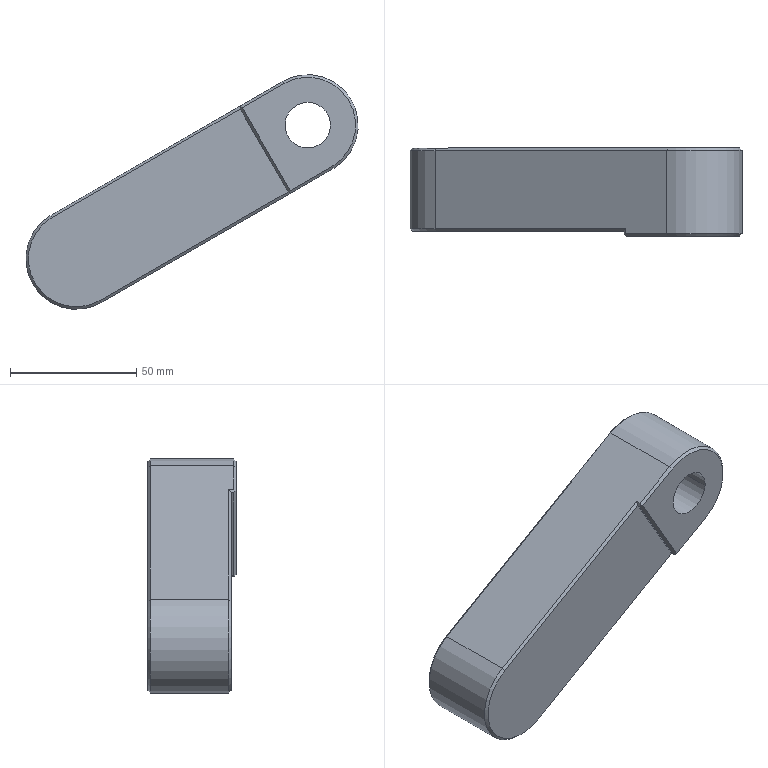Part | Creo | 1 solid | 26 faces | box 131.799 x 35 x 93 mm | volume 169707 mm3 | plane 16 | cylinder 6 | cone 4 | commonest cylinder face diameters 18.05 x2 26 x2 40 x2
STEP:
#1=CARTESIAN_POINT('',(-32.067,331.995,-173.29));
#2=VERTEX_POINT('',#1);
#3=CARTESIAN_POINT('',(-32.067,347.995,-173.29));
#4=VERTEX_POINT('',#3);
#5=CARTESIAN_POINT('',(-32.067,331.995,-173.29));
#6=DIRECTION('',(0.,1.,0.));
#7=VECTOR('',#6,16.);
#8=LINE('',#5,#7);
#9=EDGE_CURVE('',#2,#4,#8,.T.);
#10=ORIENTED_EDGE('',*,*,#9,.T.);
#11=CARTESIAN_POINT('',(-14.085,347.995,-174.863));
#12=VERTEX_POINT('',#11);
#13=CARTESIAN_POINT('',(-23.076,347.995,-174.076));
#14=DIRECTION('',(0.,-1.,0.));
#15=DIRECTION('',(-0.9962,0.,0.08716));
#16=AXIS2_PLACEMENT_3D('',#13,#14,#15);
#17=CIRCLE('',#16,9.025);
#18=EDGE_CURVE('',#4,#12,#17,.T.);
#19=ORIENTED_EDGE('',*,*,#18,.T.);
#20=CARTESIAN_POINT('',(-14.085,331.995,-174.863));
#21=VERTEX_POINT('',#20);
#22=CARTESIAN_POINT('',(-14.085,347.995,-174.863));
#23=DIRECTION('',(0.,-1.,0.));
#24=VECTOR('',#23,16.);
#25=LINE('',#22,#24);
#26=EDGE_CURVE('',#12,#21,#25,.T.);
#27=ORIENTED_EDGE('',*,*,#26,.T.);
#28=CARTESIAN_POINT('',(-23.076,331.995,-174.076));
#29=DIRECTION('',(0.,1.,0.));
#30=DIRECTION('',(0.9962,0.,-0.08716));
#31=AXIS2_PLACEMENT_3D('',#28,#29,#30);
#32=CIRCLE('',#31,9.025);
#33=EDGE_CURVE('',#21,#2,#32,.T.);
#34=ORIENTED_EDGE('',*,*,#33,.T.);
#35=EDGE_LOOP('',(#10,#19,#27,#34));
#36=FACE_OUTER_BOUND('',#35,.F.);
#37=CARTESIAN_POINT('',(-23.076,366.995,-174.076));
#38=DIRECTION('',(0.,1.,0.));
#39=DIRECTION('',(-0.9962,0.,0.08716));
#40=AXIS2_PLACEMENT_3D('',#37,#38,#39);
#41=CYLINDRICAL_SURFACE('',#40,9.025);
#42=ADVANCED_FACE('',(#36),#41,.F.);
#43=ORIENTED_EDGE('',*,*,#26,.F.);
#44=CARTESIAN_POINT('',(-23.076,347.995,-174.076));
#45=DIRECTION('',(0.,-1.,0.));
#46=DIRECTION('',(0.9962,0.,-0.08716));
#47=AXIS2_PLACEMENT_3D('',#44,#45,#46);
#48=CIRCLE('',#47,9.025);
#49=EDGE_CURVE('',#12,#4,#48,.T.);
#50=ORIENTED_EDGE('',*,*,#49,.T.);
#51=ORIENTED_EDGE('',*,*,#9,.F.);
#52=CARTESIAN_POINT('',(-23.076,331.995,-174.076));
#53=DIRECTION('',(0.,1.,0.));
#54=DIRECTION('',(-0.9962,0.,0.08716));
#55=AXIS2_PLACEMENT_3D('',#52,#53,#54);
#56=CIRCLE('',#55,9.025);
#57=EDGE_CURVE('',#2,#21,#56,.T.);
#58=ORIENTED_EDGE('',*,*,#57,.T.);
#59=EDGE_LOOP('',(#43,#50,#51,#58));
#60=FACE_OUTER_BOUND('',#59,.F.);
#61=CARTESIAN_POINT('',(-23.076,366.995,-174.076));
#62=DIRECTION('',(0.,1.,0.));
#63=DIRECTION('',(-0.9962,0.,0.08716));
#64=AXIS2_PLACEMENT_3D('',#61,#62,#63);
#65=CYLINDRICAL_SURFACE('',#64,9.025);
#66=ADVANCED_FACE('',(#60),#65,.F.);
#67=CARTESIAN_POINT('',(-10.126,347.995,-175.209));
#68=VERTEX_POINT('',#67);
#69=CARTESIAN_POINT('',(-36.027,347.995,-172.943));
#70=VERTEX_POINT('',#69);
#71=CARTESIAN_POINT('',(-23.076,347.995,-174.076));
#72=DIRECTION('',(0.,1.,0.));
#73=DIRECTION('',(0.9962,0.,-0.08716));
#74=AXIS2_PLACEMENT_3D('',#71,#72,#73);
#75=CIRCLE('',#74,13.);
#76=EDGE_CURVE('',#68,#70,#75,.T.);
#77=ORIENTED_EDGE('',*,*,#76,.F.);
#78=CARTESIAN_POINT('',(-23.076,347.995,-174.076));
#79=DIRECTION('',(0.,1.,0.));
#80=DIRECTION('',(-0.9962,0.,0.08716));
#81=AXIS2_PLACEMENT_3D('',#78,#79,#80);
#82=CIRCLE('',#81,13.);
#83=EDGE_CURVE('',#70,#68,#82,.T.);
#84=ORIENTED_EDGE('',*,*,#83,.F.);
#85=EDGE_LOOP('',(#77,#84));
#86=FACE_OUTER_BOUND('',#85,.F.);
#87=ORIENTED_EDGE('',*,*,#18,.F.);
#88=ORIENTED_EDGE('',*,*,#49,.F.);
#89=EDGE_LOOP('',(#87,#88));
#90=FACE_BOUND('',#89,.F.);
#91=CARTESIAN_POINT('',(-167.611,347.995,-30.602));
#92=DIRECTION('',(0.,1.,0.));
#93=DIRECTION('',(-0.9962,0.,0.08716));
#94=AXIS2_PLACEMENT_3D('',#91,#92,#93);
#95=PLANE('',#94);
#96=ADVANCED_FACE('',(#86,#90),#95,.T.);
#97=CARTESIAN_POINT('',(-36.027,366.995,-172.943));
#98=VERTEX_POINT('',#97);
#99=CARTESIAN_POINT('',(-36.027,347.995,-172.943));
#100=DIRECTION('',(0.,1.,0.));
#101=VECTOR('',#100,19.);
#102=LINE('',#99,#101);
#103=EDGE_CURVE('',#70,#98,#102,.T.);
#104=ORIENTED_EDGE('',*,*,#103,.T.);
#105=CARTESIAN_POINT('',(-10.126,366.995,-175.209));
#106=VERTEX_POINT('',#105);
#107=CARTESIAN_POINT('',(-23.076,366.995,-174.076));
#108=DIRECTION('',(0.,-1.,0.));
#109=DIRECTION('',(-0.9962,0.,0.08716));
#110=AXIS2_PLACEMENT_3D('',#107,#108,#109);
#111=CIRCLE('',#110,13.);
#112=EDGE_CURVE('',#98,#106,#111,.T.);
#113=ORIENTED_EDGE('',*,*,#112,.T.);
#114=CARTESIAN_POINT('',(-10.126,366.995,-175.209));
#115=DIRECTION('',(0.,-1.,0.));
#116=VECTOR('',#115,19.);
#117=LINE('',#114,#116);
#118=EDGE_CURVE('',#106,#68,#117,.T.);
#119=ORIENTED_EDGE('',*,*,#118,.T.);
#120=ORIENTED_EDGE('',*,*,#76,.T.);
#121=EDGE_LOOP('',(#104,#113,#119,#120));
#122=FACE_OUTER_BOUND('',#121,.F.);
#123=CARTESIAN_POINT('',(-23.076,366.995,-174.076));
#124=DIRECTION('',(0.,1.,0.));
#125=DIRECTION('',(-0.9962,0.,0.08716));
#126=AXIS2_PLACEMENT_3D('',#123,#124,#125);
#127=CYLINDRICAL_SURFACE('',#126,13.);
#128=ADVANCED_FACE('',(#122),#127,.F.);
#129=ORIENTED_EDGE('',*,*,#118,.F.);
#130=CARTESIAN_POINT('',(-23.076,366.995,-174.076));
#131=DIRECTION('',(0.,-1.,0.));
#132=DIRECTION('',(0.9962,0.,-0.08716));
#133=AXIS2_PLACEMENT_3D('',#130,#131,#132);
#134=CIRCLE('',#133,13.);
#135=EDGE_CURVE('',#106,#98,#134,.T.);
#136=ORIENTED_EDGE('',*,*,#135,.T.);
#137=ORIENTED_EDGE('',*,*,#103,.F.);
#138=ORIENTED_EDGE('',*,*,#83,.T.);
#139=EDGE_LOOP('',(#129,#136,#137,#138));
#140=FACE_OUTER_BOUND('',#139,.F.);
#141=CARTESIAN_POINT('',(-23.076,366.995,-174.076));
#142=DIRECTION('',(0.,1.,0.));
#143=DIRECTION('',(-0.9962,0.,0.08716));
#144=AXIS2_PLACEMENT_3D('',#141,#142,#143);
#145=CYLINDRICAL_SURFACE('',#144,13.);
#146=ADVANCED_FACE('',(#140),#145,.F.);
#147=CARTESIAN_POINT('',(-124.375,366.995,-210.622));
#148=VERTEX_POINT('',#147);
#149=CARTESIAN_POINT('',(-32.576,366.995,-157.622));
#150=VERTEX_POINT('',#149);
#151=CARTESIAN_POINT('',(-124.375,366.995,-210.622));
#152=DIRECTION('',(0.866,0.,0.5));
#153=VECTOR('',#152,106.);
#154=LINE('',#151,#153);
#155=EDGE_CURVE('',#148,#150,#154,.T.);
#156=ORIENTED_EDGE('',*,*,#155,.F.);
#157=CARTESIAN_POINT('',(-119.792,366.995,-245.429));
#158=VERTEX_POINT('',#157);
#159=CARTESIAN_POINT('',(-114.875,366.995,-227.076));
#160=DIRECTION('',(0.,1.,0.));
#161=DIRECTION('',(-0.2588,0.,-0.9659));
#162=AXIS2_PLACEMENT_3D('',#159,#160,#161);
#163=CIRCLE('',#162,19.);
#164=EDGE_CURVE('',#158,#148,#163,.T.);
#165=ORIENTED_EDGE('',*,*,#164,.F.);
#166=CARTESIAN_POINT('',(-116.531,366.995,-246.004));
#167=VERTEX_POINT('',#166);
#168=CARTESIAN_POINT('',(-114.875,366.995,-227.076));
#169=DIRECTION('',(0.,1.,0.));
#170=DIRECTION('',(-0.08716,0.,-0.9962));
#171=AXIS2_PLACEMENT_3D('',#168,#169,#170);
#172=CIRCLE('',#171,19.);
#173=EDGE_CURVE('',#167,#158,#172,.T.);
#174=ORIENTED_EDGE('',*,*,#173,.F.);
#175=CARTESIAN_POINT('',(-105.375,366.995,-243.531));
#176=VERTEX_POINT('',#175);
#177=CARTESIAN_POINT('',(-114.875,366.995,-227.076));
#178=DIRECTION('',(0.,1.,0.));
#179=DIRECTION('',(0.5,0.,-0.866));
#180=AXIS2_PLACEMENT_3D('',#177,#178,#179);
#181=CIRCLE('',#180,19.);
#182=EDGE_CURVE('',#176,#167,#181,.T.);
#183=ORIENTED_EDGE('',*,*,#182,.F.);
#184=CARTESIAN_POINT('',(-13.576,366.995,-190.531));
#185=VERTEX_POINT('',#184);
#186=CARTESIAN_POINT('',(-13.576,366.995,-190.531));
#187=DIRECTION('',(-0.866,0.,-0.5));
#188=VECTOR('',#187,106.);
#189=LINE('',#186,#188);
#190=EDGE_CURVE('',#185,#176,#189,.T.);
#191=ORIENTED_EDGE('',*,*,#190,.F.);
#192=CARTESIAN_POINT('',(-21.42,366.995,-155.148));
#193=VERTEX_POINT('',#192);
#194=CARTESIAN_POINT('',(-23.076,366.995,-174.076));
#195=DIRECTION('',(0.,1.,0.));
#196=DIRECTION('',(0.08716,0.,0.9962));
#197=AXIS2_PLACEMENT_3D('',#194,#195,#196);
#198=CIRCLE('',#197,19.);
#199=EDGE_CURVE('',#193,#185,#198,.T.);
#200=ORIENTED_EDGE('',*,*,#199,.F.);
#201=CARTESIAN_POINT('',(-23.076,366.995,-174.076));
#202=DIRECTION('',(0.,1.,0.));
#203=DIRECTION('',(-0.5,0.,0.866));
#204=AXIS2_PLACEMENT_3D('',#201,#202,#203);
#205=CIRCLE('',#204,19.);
#206=EDGE_CURVE('',#150,#193,#205,.T.);
#207=ORIENTED_EDGE('',*,*,#206,.F.);
#208=EDGE_LOOP('',(#156,#165,#174,#183,#191,#200,#207));
#209=FACE_OUTER_BOUND('',#208,.F.);
#210=ORIENTED_EDGE('',*,*,#112,.F.);
#211=ORIENTED_EDGE('',*,*,#135,.F.);
#212=EDGE_LOOP('',(#210,#211));
#213=FACE_BOUND('',#212,.F.);
#214=CARTESIAN_POINT('',(-167.611,366.995,-30.602));
#215=DIRECTION('',(0.,1.,0.));
#216=DIRECTION('',(-0.9962,0.,0.08716));
#217=AXIS2_PLACEMENT_3D('',#214,#215,#216);
#218=PLANE('',#217);
#219=ADVANCED_FACE('',(#209,#213),#218,.T.);
#220=CARTESIAN_POINT('',(-124.875,365.995,-209.756));
#221=VERTEX_POINT('',#220);
#222=CARTESIAN_POINT('',(-124.875,365.995,-209.756));
#223=DIRECTION('',(0.3536,0.7071,-0.6124));
#224=VECTOR('',#223,1.414);
#225=LINE('',#222,#224);
#226=EDGE_CURVE('',#221,#148,#225,.T.);
#227=ORIENTED_EDGE('',*,*,#226,.T.);
#228=ORIENTED_EDGE('',*,*,#155,.T.);
#229=CARTESIAN_POINT('',(-33.076,365.995,-156.756));
#230=VERTEX_POINT('',#229);
#231=CARTESIAN_POINT('',(-32.576,366.995,-157.622));
#232=DIRECTION('',(-0.3536,-0.7071,0.6124));
#233=VECTOR('',#232,1.414);
#234=LINE('',#231,#233);
#235=EDGE_CURVE('',#150,#230,#234,.T.);
#236=ORIENTED_EDGE('',*,*,#235,.T.);
#237=CARTESIAN_POINT('',(-33.076,365.995,-156.756));
#238=DIRECTION('',(-0.866,0.,-0.5));
#239=VECTOR('',#238,106.);
#240=LINE('',#237,#239);
#241=EDGE_CURVE('',#230,#221,#240,.T.);
#242=ORIENTED_EDGE('',*,*,#241,.T.);
#243=EDGE_LOOP('',(#227,#228,#236,#242));
#244=FACE_OUTER_BOUND('',#243,.F.);
#245=CARTESIAN_POINT('',(-89.118,366.495,-189.689));
#246=DIRECTION('',(-0.3536,0.7071,0.6124));
#247=DIRECTION('',(-0.3536,-0.7071,0.6124));
#248=AXIS2_PLACEMENT_3D('',#245,#246,#247);
#249=PLANE('',#248);
#250=ADVANCED_FACE('',(#244),#249,.T.);
#251=CARTESIAN_POINT('',(-104.875,365.995,-244.397));
#252=VERTEX_POINT('',#251);
#253=CARTESIAN_POINT('',(-105.375,366.995,-243.531));
#254=DIRECTION('',(0.3536,-0.7071,-0.6124));
#255=VECTOR('',#254,1.414);
#256=LINE('',#253,#255);
#257=EDGE_CURVE('',#176,#252,#256,.T.);
#258=ORIENTED_EDGE('',*,*,#257,.F.);
#259=ORIENTED_EDGE('',*,*,#182,.T.);
#260=ORIENTED_EDGE('',*,*,#173,.T.);
#261=ORIENTED_EDGE('',*,*,#164,.T.);
#262=ORIENTED_EDGE('',*,*,#226,.F.);
#263=CARTESIAN_POINT('',(-134.799,365.995,-225.333));
#264=VERTEX_POINT('',#263);
#265=CARTESIAN_POINT('',(-114.875,365.995,-227.076));
#266=DIRECTION('',(0.,1.,0.));
#267=DIRECTION('',(-0.9962,0.,0.08716));
#268=AXIS2_PLACEMENT_3D('',#265,#266,#267);
#269=CIRCLE('',#268,20.);
#270=EDGE_CURVE('',#264,#221,#269,.T.);
#271=ORIENTED_EDGE('',*,*,#270,.F.);
#272=CARTESIAN_POINT('',(-116.618,365.995,-247.));
#273=VERTEX_POINT('',#272);
#274=CARTESIAN_POINT('',(-114.875,365.995,-227.076));
#275=DIRECTION('',(0.,1.,0.));
#276=DIRECTION('',(-0.08716,0.,-0.9962));
#277=AXIS2_PLACEMENT_3D('',#274,#275,#276);
#278=CIRCLE('',#277,20.);
#279=EDGE_CURVE('',#273,#264,#278,.T.);
#280=ORIENTED_EDGE('',*,*,#279,.F.);
#281=CARTESIAN_POINT('',(-114.875,365.995,-227.076));
#282=DIRECTION('',(0.,1.,0.));
#283=DIRECTION('',(0.5,0.,-0.866));
#284=AXIS2_PLACEMENT_3D('',#281,#282,#283);
#285=CIRCLE('',#284,20.);
#286=EDGE_CURVE('',#252,#273,#285,.T.);
#287=ORIENTED_EDGE('',*,*,#286,.F.);
#288=EDGE_LOOP('',(#258,#259,#260,#261,#262,#271,#280,#287));
#289=FACE_OUTER_BOUND('',#288,.F.);
#290=CARTESIAN_POINT('',(-114.875,366.495,-227.076));
#291=DIRECTION('',(0.,-1.,0.));
#292=DIRECTION('',(-0.08716,0.,-0.9962));
#293=AXIS2_PLACEMENT_3D('',#290,#291,#292);
#294=CONICAL_SURFACE('',#293,19.5,45.);
#295=ADVANCED_FACE('',(#289),#294,.T.);
#296=CARTESIAN_POINT('',(-13.076,365.995,-191.397));
#297=VERTEX_POINT('',#296);
#298=CARTESIAN_POINT('',(-13.076,365.995,-191.397));
#299=DIRECTION('',(-0.3536,0.7071,0.6124));
#300=VECTOR('',#299,1.414);
#301=LINE('',#298,#300);
#302=EDGE_CURVE('',#297,#185,#301,.T.);
#303=ORIENTED_EDGE('',*,*,#302,.T.);
#304=ORIENTED_EDGE('',*,*,#190,.T.);
#305=ORIENTED_EDGE('',*,*,#257,.T.);
#306=CARTESIAN_POINT('',(-104.875,365.995,-244.397));
#307=DIRECTION('',(0.866,0.,0.5));
#308=VECTOR('',#307,106.);
#309=LINE('',#306,#308);
#310=EDGE_CURVE('',#252,#297,#309,.T.);
#311=ORIENTED_EDGE('',*,*,#310,.T.);
#312=EDGE_LOOP('',(#303,#304,#305,#311));
#313=FACE_OUTER_BOUND('',#312,.F.);
#314=CARTESIAN_POINT('',(-69.618,366.495,-223.464));
#315=DIRECTION('',(0.3536,0.7071,-0.6124));
#316=DIRECTION('',(0.3536,-0.7071,-0.6124));
#317=AXIS2_PLACEMENT_3D('',#314,#315,#316);
#318=PLANE('',#317);
#319=ADVANCED_FACE('',(#313),#318,.T.);
#320=ORIENTED_EDGE('',*,*,#235,.F.);
#321=ORIENTED_EDGE('',*,*,#206,.T.);
#322=ORIENTED_EDGE('',*,*,#199,.T.);
#323=ORIENTED_EDGE('',*,*,#302,.F.);
#324=CARTESIAN_POINT('',(-3.152,365.995,-175.819));
#325=VERTEX_POINT('',#324);
#326=CARTESIAN_POINT('',(-23.076,365.995,-174.076));
#327=DIRECTION('',(0.,1.,0.));
#328=DIRECTION('',(0.9962,0.,-0.08716));
#329=AXIS2_PLACEMENT_3D('',#326,#327,#328);
#330=CIRCLE('',#329,20.);
#331=EDGE_CURVE('',#325,#297,#330,.T.);
#332=ORIENTED_EDGE('',*,*,#331,.F.);
#333=CARTESIAN_POINT('',(-21.333,365.995,-154.152));
#334=VERTEX_POINT('',#333);
#335=CARTESIAN_POINT('',(-23.076,365.995,-174.076));
#336=DIRECTION('',(0.,1.,0.));
#337=DIRECTION('',(0.08716,0.,0.9962));
#338=AXIS2_PLACEMENT_3D('',#335,#336,#337);
#339=CIRCLE('',#338,20.);
#340=EDGE_CURVE('',#334,#325,#339,.T.);
#341=ORIENTED_EDGE('',*,*,#340,.F.);
#342=CARTESIAN_POINT('',(-23.076,365.995,-174.076));
#343=DIRECTION('',(0.,1.,0.));
#344=DIRECTION('',(-0.5,0.,0.866));
#345=AXIS2_PLACEMENT_3D('',#342,#343,#344);
#346=CIRCLE('',#345,20.);
#347=EDGE_CURVE('',#230,#334,#346,.T.);
#348=ORIENTED_EDGE('',*,*,#347,.F.);
#349=EDGE_LOOP('',(#320,#321,#322,#323,#332,#341,#348));
#350=FACE_OUTER_BOUND('',#349,.F.);
#351=CARTESIAN_POINT('',(-23.076,366.495,-174.076));
#352=DIRECTION('',(0.,-1.,0.));
#353=DIRECTION('',(-0.08716,0.,-0.9962));
#354=AXIS2_PLACEMENT_3D('',#351,#352,#353);
#355=CONICAL_SURFACE('',#354,19.5,45.);
#356=ADVANCED_FACE('',(#350),#355,.T.);
#357=CARTESIAN_POINT('',(-13.076,332.995,-191.397));
#358=VERTEX_POINT('',#357);
#359=CARTESIAN_POINT('',(-13.076,332.995,-191.397));
#360=DIRECTION('',(0.000000003,1.,0.000000002));
#361=VECTOR('',#360,33.);
#362=LINE('',#359,#361);
#363=EDGE_CURVE('',#358,#297,#362,.T.);
#364=ORIENTED_EDGE('',*,*,#363,.F.);
#365=CARTESIAN_POINT('',(-3.152,332.995,-175.819));
#366=VERTEX_POINT('',#365);
#367=CARTESIAN_POINT('',(-23.076,332.995,-174.076));
#368=DIRECTION('',(0.,-1.,0.));
#369=DIRECTION('',(0.5,0.,-0.866));
#370=AXIS2_PLACEMENT_3D('',#367,#368,#369);
#371=CIRCLE('',#370,20.);
#372=EDGE_CURVE('',#358,#366,#371,.T.);
#373=ORIENTED_EDGE('',*,*,#372,.T.);
#374=CARTESIAN_POINT('',(-21.333,332.995,-154.152));
#375=VERTEX_POINT('',#374);
#376=CARTESIAN_POINT('',(-23.076,332.995,-174.076));
#377=DIRECTION('',(0.,-1.,0.));
#378=DIRECTION('',(0.9962,0.,-0.08716));
#379=AXIS2_PLACEMENT_3D('',#376,#377,#378);
#380=CIRCLE('',#379,20.);
#381=EDGE_CURVE('',#366,#375,#380,.T.);
#382=ORIENTED_EDGE('',*,*,#381,.T.);
#383=CARTESIAN_POINT('',(-33.076,332.995,-156.756));
#384=VERTEX_POINT('',#383);
#385=CARTESIAN_POINT('',(-23.076,332.995,-174.076));
#386=DIRECTION('',(0.,-1.,0.));
#387=DIRECTION('',(0.08716,0.,0.9962));
#388=AXIS2_PLACEMENT_3D('',#385,#386,#387);
#389=CIRCLE('',#388,20.);
#390=EDGE_CURVE('',#375,#384,#389,.T.);
#391=ORIENTED_EDGE('',*,*,#390,.T.);
#392=CARTESIAN_POINT('',(-33.076,365.995,-156.756));
#393=DIRECTION('',(-0.000000004,-1.,-0.000000002));
#394=VECTOR('',#393,33.);
#395=LINE('',#392,#394);
#396=EDGE_CURVE('',#230,#384,#395,.T.);
#397=ORIENTED_EDGE('',*,*,#396,.F.);
#398=ORIENTED_EDGE('',*,*,#347,.T.);
#399=ORIENTED_EDGE('',*,*,#340,.T.);
#400=ORIENTED_EDGE('',*,*,#331,.T.);
#401=EDGE_LOOP('',(#364,#373,#382,#391,#397,#398,#399,#400));
#402=FACE_OUTER_BOUND('',#401,.F.);
#403=CARTESIAN_POINT('',(-23.076,331.995,-174.076));
#404=DIRECTION('',(0.,1.,0.));
#405=DIRECTION('',(-0.9962,0.,0.08716));
#406=AXIS2_PLACEMENT_3D('',#403,#404,#405);
#407=CYLINDRICAL_SURFACE('',#406,20.);
#408=ADVANCED_FACE('',(#402),#407,.T.);
#409=CARTESIAN_POINT('',(-104.875,334.995,-244.397));
#410=VERTEX_POINT('',#409);
#411=CARTESIAN_POINT('',(-104.875,365.995,-244.397));
#412=DIRECTION('',(0.,-1.,0.));
#413=VECTOR('',#412,31.);
#414=LINE('',#411,#413);
#415=EDGE_CURVE('',#252,#410,#414,.T.);
#416=ORIENTED_EDGE('',*,*,#415,.T.);
#417=CARTESIAN_POINT('',(-29.531,334.995,-200.897));
#418=VERTEX_POINT('',#417);
#419=CARTESIAN_POINT('',(-104.875,334.995,-244.397));
#420=DIRECTION('',(0.866,0.,0.5));
#421=VECTOR('',#420,87.);
#422=LINE('',#419,#421);
#423=EDGE_CURVE('',#410,#418,#422,.T.);
#424=ORIENTED_EDGE('',*,*,#423,.T.);
#425=CARTESIAN_POINT('',(-29.531,332.995,-200.897));
#426=VERTEX_POINT('',#425);
#427=CARTESIAN_POINT('',(-29.531,334.995,-200.897));
#428=DIRECTION('',(0.,-1.,0.));
#429=VECTOR('',#428,2.);
#430=LINE('',#427,#429);
#431=EDGE_CURVE('',#418,#426,#430,.T.);
#432=ORIENTED_EDGE('',*,*,#431,.T.);
#433=CARTESIAN_POINT('',(-13.076,332.995,-191.397));
#434=DIRECTION('',(-0.866,0.,-0.5));
#435=VECTOR('',#434,19.);
#436=LINE('',#433,#435);
#437=EDGE_CURVE('',#358,#426,#436,.T.);
#438=ORIENTED_EDGE('',*,*,#437,.F.);
#439=ORIENTED_EDGE('',*,*,#363,.T.);
#440=ORIENTED_EDGE('',*,*,#310,.F.);
#441=EDGE_LOOP('',(#416,#424,#432,#438,#439,#440));
#442=FACE_OUTER_BOUND('',#441,.F.);
#443=CARTESIAN_POINT('',(-13.076,331.995,-191.397));
#444=DIRECTION('',(0.5,0.,-0.866));
#445=DIRECTION('',(-0.866,0.,-0.5));
#446=AXIS2_PLACEMENT_3D('',#443,#444,#445);
#447=PLANE('',#446);
#448=ADVANCED_FACE('',(#442),#447,.T.);
#449=CARTESIAN_POINT('',(-124.875,334.995,-209.756));
#450=VERTEX_POINT('',#449);
#451=CARTESIAN_POINT('',(-124.875,334.995,-209.756));
#452=DIRECTION('',(0.,1.,0.));
#453=VECTOR('',#452,31.);
#454=LINE('',#451,#453);
#455=EDGE_CURVE('',#450,#221,#454,.T.);
#456=ORIENTED_EDGE('',*,*,#455,.F.);
#457=CARTESIAN_POINT('',(-134.799,334.995,-225.333));
#458=VERTEX_POINT('',#457);
#459=CARTESIAN_POINT('',(-114.875,334.995,-227.076));
#460=DIRECTION('',(0.,-1.,0.));
#461=DIRECTION('',(-0.5,0.,0.866));
#462=AXIS2_PLACEMENT_3D('',#459,#460,#461);
#463=CIRCLE('',#462,20.);
#464=EDGE_CURVE('',#450,#458,#463,.T.);
#465=ORIENTED_EDGE('',*,*,#464,.T.);
#466=CARTESIAN_POINT('',(-116.618,334.995,-247.));
#467=VERTEX_POINT('',#466);
#468=CARTESIAN_POINT('',(-114.875,334.995,-227.076));
#469=DIRECTION('',(0.,-1.,0.));
#470=DIRECTION('',(-0.9962,0.,0.08716));
#471=AXIS2_PLACEMENT_3D('',#468,#469,#470);
#472=CIRCLE('',#471,20.);
#473=EDGE_CURVE('',#458,#467,#472,.T.);
#474=ORIENTED_EDGE('',*,*,#473,.T.);
#475=CARTESIAN_POINT('',(-114.875,334.995,-227.076));
#476=DIRECTION('',(0.,-1.,0.));
#477=DIRECTION('',(-0.08716,0.,-0.9962));
#478=AXIS2_PLACEMENT_3D('',#475,#476,#477);
#479=CIRCLE('',#478,20.);
#480=EDGE_CURVE('',#467,#410,#479,.T.);
#481=ORIENTED_EDGE('',*,*,#480,.T.);
#482=ORIENTED_EDGE('',*,*,#415,.F.);
#483=ORIENTED_EDGE('',*,*,#286,.T.);
#484=ORIENTED_EDGE('',*,*,#279,.T.);
#485=ORIENTED_EDGE('',*,*,#270,.T.);
#486=EDGE_LOOP('',(#456,#465,#474,#481,#482,#483,#484,#485));
#487=FACE_OUTER_BOUND('',#486,.F.);
#488=CARTESIAN_POINT('',(-114.875,331.995,-227.076));
#489=DIRECTION('',(0.,1.,0.));
#490=DIRECTION('',(-0.9962,0.,0.08716));
#491=AXIS2_PLACEMENT_3D('',#488,#489,#490);
#492=CYLINDRICAL_SURFACE('',#491,20.);
#493=ADVANCED_FACE('',(#487),#492,.T.);
#494=CARTESIAN_POINT('',(-49.531,332.995,-166.256));
#495=VERTEX_POINT('',#494);
#496=CARTESIAN_POINT('',(-49.531,332.995,-166.256));
#497=DIRECTION('',(0.866,0.,0.5));
#498=VECTOR('',#497,19.);
#499=LINE('',#496,#498);
#500=EDGE_CURVE('',#495,#384,#499,.T.);
#501=ORIENTED_EDGE('',*,*,#500,.F.);
#502=CARTESIAN_POINT('',(-49.531,334.995,-166.256));
#503=VERTEX_POINT('',#502);
#504=CARTESIAN_POINT('',(-49.531,332.995,-166.256));
#505=DIRECTION('',(0.,1.,0.));
#506=VECTOR('',#505,2.);
#507=LINE('',#504,#506);
#508=EDGE_CURVE('',#495,#503,#507,.T.);
#509=ORIENTED_EDGE('',*,*,#508,.T.);
#510=CARTESIAN_POINT('',(-49.531,334.995,-166.256));
#511=DIRECTION('',(-0.866,0.,-0.5));
#512=VECTOR('',#511,87.);
#513=LINE('',#510,#512);
#514=EDGE_CURVE('',#503,#450,#513,.T.);
#515=ORIENTED_EDGE('',*,*,#514,.T.);
#516=ORIENTED_EDGE('',*,*,#455,.T.);
#517=ORIENTED_EDGE('',*,*,#241,.F.);
#518=ORIENTED_EDGE('',*,*,#396,.T.);
#519=EDGE_LOOP('',(#501,#509,#515,#516,#517,#518));
#520=FACE_OUTER_BOUND('',#519,.F.);
#521=CARTESIAN_POINT('',(-145.659,331.995,-221.756));
#522=DIRECTION('',(-0.5,0.,0.866));
#523=DIRECTION('',(0.866,0.,0.5));
#524=AXIS2_PLACEMENT_3D('',#521,#522,#523);
#525=PLANE('',#524);
#526=ADVANCED_FACE('',(#520),#525,.T.);
#527=CARTESIAN_POINT('',(-49.714,332.495,-166.939));
#528=VERTEX_POINT('',#527);
#529=CARTESIAN_POINT('',(-49.531,332.995,-166.256));
#530=DIRECTION('',(-0.2113,-0.5774,-0.7887));
#531=VECTOR('',#530,0.866);
#532=LINE('',#529,#531);
#533=EDGE_CURVE('',#495,#528,#532,.T.);
#534=ORIENTED_EDGE('',*,*,#533,.F.);
#535=ORIENTED_EDGE('',*,*,#500,.T.);
#536=CARTESIAN_POINT('',(-32.576,331.995,-157.622));
#537=VERTEX_POINT('',#536);
#538=CARTESIAN_POINT('',(-33.076,332.995,-156.756));
#539=DIRECTION('',(0.3536,-0.7071,-0.6124));
#540=VECTOR('',#539,1.414);
#541=LINE('',#538,#540);
#542=EDGE_CURVE('',#384,#537,#541,.T.);
#543=ORIENTED_EDGE('',*,*,#542,.T.);
#544=CARTESIAN_POINT('',(-49.031,331.995,-167.122));
#545=VERTEX_POINT('',#544);
#546=CARTESIAN_POINT('',(-32.576,331.995,-157.622));
#547=DIRECTION('',(-0.866,0.,-0.5));
#548=VECTOR('',#547,19.);
#549=LINE('',#546,#548);
#550=EDGE_CURVE('',#537,#545,#549,.T.);
#551=ORIENTED_EDGE('',*,*,#550,.T.);
#552=CARTESIAN_POINT('',(-49.714,332.495,-166.939));
#553=DIRECTION('',(0.7887,-0.5774,-0.2113));
#554=VECTOR('',#553,0.866);
#555=LINE('',#552,#554);
#556=EDGE_CURVE('',#528,#545,#555,.T.);
#557=ORIENTED_EDGE('',*,*,#556,.F.);
#558=EDGE_LOOP('',(#534,#535,#543,#551,#557));
#559=FACE_OUTER_BOUND('',#558,.F.);
#560=CARTESIAN_POINT('',(-41.486,332.495,-162.189));
#561=DIRECTION('',(-0.3536,-0.7071,0.6124));
#562=DIRECTION('',(-0.3536,0.7071,0.6124));
#563=AXIS2_PLACEMENT_3D('',#560,#561,#562);
#564=PLANE('',#563);
#565=ADVANCED_FACE('',(#559),#564,.T.);
#566=CARTESIAN_POINT('',(-49.897,333.995,-167.622));
#567=VERTEX_POINT('',#566);
#568=CARTESIAN_POINT('',(-49.531,334.995,-166.256));
#569=DIRECTION('',(-0.2113,-0.5774,-0.7887));
#570=VECTOR('',#569,1.732);
#571=LINE('',#568,#570);
#572=EDGE_CURVE('',#503,#567,#571,.T.);
#573=ORIENTED_EDGE('',*,*,#572,.F.);
#574=ORIENTED_EDGE('',*,*,#508,.F.);
#575=ORIENTED_EDGE('',*,*,#533,.T.);
#576=CARTESIAN_POINT('',(-49.897,332.995,-167.622));
#577=VERTEX_POINT('',#576);
#578=CARTESIAN_POINT('',(-49.714,332.495,-166.939));
#579=DIRECTION('',(-0.2113,0.5774,-0.7887));
#580=VECTOR('',#579,0.866);
#581=LINE('',#578,#580);
#582=EDGE_CURVE('',#528,#577,#581,.T.);
#583=ORIENTED_EDGE('',*,*,#582,.T.);
#584=CARTESIAN_POINT('',(-49.897,332.995,-167.622));
#585=DIRECTION('',(0.,1.,0.));
#586=VECTOR('',#585,1.);
#587=LINE('',#584,#586);
#588=EDGE_CURVE('',#577,#567,#587,.T.);
#589=ORIENTED_EDGE('',*,*,#588,.T.);
#590=EDGE_LOOP('',(#573,#574,#575,#583,#589));
#591=FACE_OUTER_BOUND('',#590,.F.);
#592=CARTESIAN_POINT('',(-49.714,332.995,-166.939));
#593=DIRECTION('',(-0.9659,0.,0.2588));
#594=DIRECTION('',(-0.2588,0.,-0.9659));
#595=AXIS2_PLACEMENT_3D('',#592,#593,#594);
#596=PLANE('',#595);
#597=ADVANCED_FACE('',(#591),#596,.T.);
#598=ORIENTED_EDGE('',*,*,#572,.T.);
#599=CARTESIAN_POINT('',(-124.375,333.995,-210.622));
#600=VERTEX_POINT('',#599);
#601=CARTESIAN_POINT('',(-49.897,333.995,-167.622));
#602=DIRECTION('',(-0.866,0.,-0.5));
#603=VECTOR('',#602,86.);
#604=LINE('',#601,#603);
#605=EDGE_CURVE('',#567,#600,#604,.T.);
#606=ORIENTED_EDGE('',*,*,#605,.T.);
#607=CARTESIAN_POINT('',(-124.375,333.995,-210.622));
#608=DIRECTION('',(-0.3536,0.7071,0.6124));
#609=VECTOR('',#608,1.414);
#610=LINE('',#607,#609);
#611=EDGE_CURVE('',#600,#450,#610,.T.);
#612=ORIENTED_EDGE('',*,*,#611,.T.);
#613=ORIENTED_EDGE('',*,*,#514,.F.);
#614=EDGE_LOOP('',(#598,#606,#612,#613));
#615=FACE_OUTER_BOUND('',#614,.F.);
#616=CARTESIAN_POINT('',(-97.778,334.495,-194.689));
#617=DIRECTION('',(-0.3536,-0.7071,0.6124));
#618=DIRECTION('',(0.3536,-0.7071,-0.6124));
#619=AXIS2_PLACEMENT_3D('',#616,#617,#618);
#620=PLANE('',#619);
#621=ADVANCED_FACE('',(#615),#620,.T.);
#622=CARTESIAN_POINT('',(-30.897,333.995,-200.531));
#623=VERTEX_POINT('',#622);
#624=CARTESIAN_POINT('',(-30.897,333.995,-200.531));
#625=DIRECTION('',(-0.5,0.,0.866));
#626=VECTOR('',#625,38.);
#627=LINE('',#624,#626);
#628=EDGE_CURVE('',#623,#567,#627,.T.);
#629=ORIENTED_EDGE('',*,*,#628,.F.);
#630=CARTESIAN_POINT('',(-105.375,333.995,-243.531));
#631=VERTEX_POINT('',#630);
#632=CARTESIAN_POINT('',(-105.375,333.995,-243.531));
#633=DIRECTION('',(0.866,0.,0.5));
#634=VECTOR('',#633,86.);
#635=LINE('',#632,#634);
#636=EDGE_CURVE('',#631,#623,#635,.T.);
#637=ORIENTED_EDGE('',*,*,#636,.F.);
#638=CARTESIAN_POINT('',(-116.531,333.995,-246.004));
#639=VERTEX_POINT('',#638);
#640=CARTESIAN_POINT('',(-114.875,333.995,-227.076));
#641=DIRECTION('',(0.,-1.,0.));
#642=DIRECTION('',(-0.08716,0.,-0.9962));
#643=AXIS2_PLACEMENT_3D('',#640,#641,#642);
#644=CIRCLE('',#643,19.);
#645=EDGE_CURVE('',#639,#631,#644,.T.);
#646=ORIENTED_EDGE('',*,*,#645,.F.);
#647=CARTESIAN_POINT('',(-114.875,333.995,-227.076));
#648=DIRECTION('',(0.,-1.,0.));
#649=DIRECTION('',(-0.5,0.,0.866));
#650=AXIS2_PLACEMENT_3D('',#647,#648,#649);
#651=CIRCLE('',#650,19.);
#652=EDGE_CURVE('',#600,#639,#651,.T.);
#653=ORIENTED_EDGE('',*,*,#652,.F.);
#654=ORIENTED_EDGE('',*,*,#605,.F.);
#655=EDGE_LOOP('',(#629,#637,#646,#653,#654));
#656=FACE_OUTER_BOUND('',#655,.F.);
#657=CARTESIAN_POINT('',(-50.397,333.995,-166.756));
#658=DIRECTION('',(0.,1.,0.));
#659=DIRECTION('',(-0.866,0.,-0.5));
#660=AXIS2_PLACEMENT_3D('',#657,#658,#659);
#661=PLANE('',#660);
#662=ADVANCED_FACE('',(#656),#661,.F.);
#663=ORIENTED_EDGE('',*,*,#628,.T.);
#664=ORIENTED_EDGE('',*,*,#588,.F.);
#665=CARTESIAN_POINT('',(-30.897,332.995,-200.531));
#666=VERTEX_POINT('',#665);
#667=CARTESIAN_POINT('',(-30.897,332.995,-200.531));
#668=DIRECTION('',(-0.5,0.,0.866));
#669=VECTOR('',#668,38.);
#670=LINE('',#667,#669);
#671=EDGE_CURVE('',#666,#577,#670,.T.);
#672=ORIENTED_EDGE('',*,*,#671,.F.);
#673=CARTESIAN_POINT('',(-30.897,333.995,-200.531));
#674=DIRECTION('',(0.,-1.,0.));
#675=VECTOR('',#674,1.);
#676=LINE('',#673,#675);
#677=EDGE_CURVE('',#623,#666,#676,.T.);
#678=ORIENTED_EDGE('',*,*,#677,.F.);
#679=EDGE_LOOP('',(#663,#664,#672,#678));
#680=FACE_OUTER_BOUND('',#679,.F.);
#681=CARTESIAN_POINT('',(-50.397,331.995,-166.756));
#682=DIRECTION('',(0.866,0.,0.5));
#683=DIRECTION('',(0.,1.,0.));
#684=AXIS2_PLACEMENT_3D('',#681,#682,#683);
#685=PLANE('',#684);
#686=ADVANCED_FACE('',(#680),#685,.F.);
#687=ORIENTED_EDGE('',*,*,#671,.T.);
#688=ORIENTED_EDGE('',*,*,#582,.F.);
#689=ORIENTED_EDGE('',*,*,#556,.T.);
#690=CARTESIAN_POINT('',(-30.031,331.995,-200.031));
#691=VERTEX_POINT('',#690);
#692=CARTESIAN_POINT('',(-49.031,331.995,-167.122));
#693=DIRECTION('',(0.5,0.,-0.866));
#694=VECTOR('',#693,38.);
#695=LINE('',#692,#694);
#696=EDGE_CURVE('',#545,#691,#695,.T.);
#697=ORIENTED_EDGE('',*,*,#696,.T.);
#698=CARTESIAN_POINT('',(-30.214,332.495,-200.714));
#699=VERTEX_POINT('',#698);
#700=CARTESIAN_POINT('',(-30.031,331.995,-200.031));
#701=DIRECTION('',(-0.2113,0.5774,-0.7887));
#702=VECTOR('',#701,0.866);
#703=LINE('',#700,#702);
#704=EDGE_CURVE('',#691,#699,#703,.T.);
#705=ORIENTED_EDGE('',*,*,#704,.T.);
#706=CARTESIAN_POINT('',(-30.214,332.495,-200.714));
#707=DIRECTION('',(-0.7887,0.5774,0.2113));
#708=VECTOR('',#707,0.866);
#709=LINE('',#706,#708);
#710=EDGE_CURVE('',#699,#666,#709,.T.);
#711=ORIENTED_EDGE('',*,*,#710,.T.);
#712=EDGE_LOOP('',(#687,#688,#689,#697,#705,#711));
#713=FACE_OUTER_BOUND('',#712,.F.);
#714=CARTESIAN_POINT('',(-39.964,332.495,-183.826));
#715=DIRECTION('',(-0.6124,-0.7071,-0.3536));
#716=DIRECTION('',(-0.6124,0.7071,-0.3536));
#717=AXIS2_PLACEMENT_3D('',#714,#715,#716);
#718=PLANE('',#717);
#719=ADVANCED_FACE('',(#713),#718,.T.);
#720=ORIENTED_EDGE('',*,*,#696,.F.);
#721=ORIENTED_EDGE('',*,*,#550,.F.);
#722=CARTESIAN_POINT('',(-21.42,331.995,-155.148));
#723=VERTEX_POINT('',#722);
#724=CARTESIAN_POINT('',(-23.076,331.995,-174.076));
#725=DIRECTION('',(0.,-1.,0.));
#726=DIRECTION('',(0.08716,0.,0.9962));
#727=AXIS2_PLACEMENT_3D('',#724,#725,#726);
#728=CIRCLE('',#727,19.);
#729=EDGE_CURVE('',#723,#537,#728,.T.);
#730=ORIENTED_EDGE('',*,*,#729,.F.);
#731=CARTESIAN_POINT('',(-13.576,331.995,-190.531));
#732=VERTEX_POINT('',#731);
#733=CARTESIAN_POINT('',(-23.076,331.995,-174.076));
#734=DIRECTION('',(0.,-1.,0.));
#735=DIRECTION('',(0.5,0.,-0.866));
#736=AXIS2_PLACEMENT_3D('',#733,#734,#735);
#737=CIRCLE('',#736,19.);
#738=EDGE_CURVE('',#732,#723,#737,.T.);
#739=ORIENTED_EDGE('',*,*,#738,.F.);
#740=CARTESIAN_POINT('',(-30.031,331.995,-200.031));
#741=DIRECTION('',(0.866,0.,0.5));
#742=VECTOR('',#741,19.);
#743=LINE('',#740,#742);
#744=EDGE_CURVE('',#691,#732,#743,.T.);
#745=ORIENTED_EDGE('',*,*,#744,.F.);
#746=EDGE_LOOP('',(#720,#721,#730,#739,#745));
#747=FACE_OUTER_BOUND('',#746,.F.);
#748=ORIENTED_EDGE('',*,*,#33,.F.);
#749=ORIENTED_EDGE('',*,*,#57,.F.);
#750=EDGE_LOOP('',(#748,#749));
#751=FACE_BOUND('',#750,.F.);
#752=CARTESIAN_POINT('',(-167.611,331.995,-30.602));
#753=DIRECTION('',(0.,1.,0.));
#754=DIRECTION('',(-0.9962,0.,0.08716));
#755=AXIS2_PLACEMENT_3D('',#752,#753,#754);
#756=PLANE('',#755);
#757=ADVANCED_FACE('',(#747,#751),#756,.F.);
#758=CARTESIAN_POINT('',(-13.076,332.995,-191.397));
#759=DIRECTION('',(-0.3536,-0.7071,0.6124));
#760=VECTOR('',#759,1.414);
#761=LINE('',#758,#760);
#762=EDGE_CURVE('',#358,#732,#761,.T.);
#763=ORIENTED_EDGE('',*,*,#762,.T.);
#764=ORIENTED_EDGE('',*,*,#738,.T.);
#765=ORIENTED_EDGE('',*,*,#729,.T.);
#766=ORIENTED_EDGE('',*,*,#542,.F.);
#767=ORIENTED_EDGE('',*,*,#390,.F.);
#768=ORIENTED_EDGE('',*,*,#381,.F.);
#769=ORIENTED_EDGE('',*,*,#372,.F.);
#770=EDGE_LOOP('',(#763,#764,#765,#766,#767,#768,#769));
#771=FACE_OUTER_BOUND('',#770,.F.);
#772=CARTESIAN_POINT('',(-23.076,332.495,-174.076));
#773=DIRECTION('',(0.,1.,0.));
#774=DIRECTION('',(-0.08716,0.,-0.9962));
#775=AXIS2_PLACEMENT_3D('',#772,#773,#774);
#776=CONICAL_SURFACE('',#775,19.5,45.);
#777=ADVANCED_FACE('',(#771),#776,.T.);
#778=ORIENTED_EDGE('',*,*,#704,.F.);
#779=ORIENTED_EDGE('',*,*,#744,.T.);
#780=ORIENTED_EDGE('',*,*,#762,.F.);
#781=ORIENTED_EDGE('',*,*,#437,.T.);
#782=CARTESIAN_POINT('',(-30.214,332.495,-200.714));
#783=DIRECTION('',(0.7887,0.5774,-0.2113));
#784=VECTOR('',#783,0.866);
#785=LINE('',#782,#784);
#786=EDGE_CURVE('',#699,#426,#785,.T.);
#787=ORIENTED_EDGE('',*,*,#786,.F.);
#788=EDGE_LOOP('',(#778,#779,#780,#781,#787));
#789=FACE_OUTER_BOUND('',#788,.F.);
#790=CARTESIAN_POINT('',(-21.986,332.495,-195.964));
#791=DIRECTION('',(0.3536,-0.7071,-0.6124));
#792=DIRECTION('',(0.3536,0.7071,-0.6124));
#793=AXIS2_PLACEMENT_3D('',#790,#791,#792);
#794=PLANE('',#793);
#795=ADVANCED_FACE('',(#789),#794,.T.);
#796=CARTESIAN_POINT('',(-29.531,334.995,-200.897));
#797=DIRECTION('',(-0.7887,-0.5774,0.2113));
#798=VECTOR('',#797,1.732);
#799=LINE('',#796,#798);
#800=EDGE_CURVE('',#418,#623,#799,.T.);
#801=ORIENTED_EDGE('',*,*,#800,.T.);
#802=ORIENTED_EDGE('',*,*,#677,.T.);
#803=ORIENTED_EDGE('',*,*,#710,.F.);
#804=ORIENTED_EDGE('',*,*,#786,.T.);
#805=ORIENTED_EDGE('',*,*,#431,.F.);
#806=EDGE_LOOP('',(#801,#802,#803,#804,#805));
#807=FACE_OUTER_BOUND('',#806,.F.);
#808=CARTESIAN_POINT('',(-30.214,332.995,-200.714));
#809=DIRECTION('',(-0.2588,0.,-0.9659));
#810=DIRECTION('',(-0.9659,0.,0.2588));
#811=AXIS2_PLACEMENT_3D('',#808,#809,#810);
#812=PLANE('',#811);
#813=ADVANCED_FACE('',(#807),#812,.T.);
#814=ORIENTED_EDGE('',*,*,#800,.F.);
#815=ORIENTED_EDGE('',*,*,#423,.F.);
#816=CARTESIAN_POINT('',(-104.875,334.995,-244.397));
#817=DIRECTION('',(-0.3536,-0.7071,0.6124));
#818=VECTOR('',#817,1.414);
#819=LINE('',#816,#818);
#820=EDGE_CURVE('',#410,#631,#819,.T.);
#821=ORIENTED_EDGE('',*,*,#820,.T.);
#822=ORIENTED_EDGE('',*,*,#636,.T.);
#823=EDGE_LOOP('',(#814,#815,#821,#822));
#824=FACE_OUTER_BOUND('',#823,.F.);
#825=CARTESIAN_POINT('',(-78.278,334.495,-228.464));
#826=DIRECTION('',(0.3536,-0.7071,-0.6124));
#827=DIRECTION('',(-0.3536,-0.7071,0.6124));
#828=AXIS2_PLACEMENT_3D('',#825,#826,#827);
#829=PLANE('',#828);
#830=ADVANCED_FACE('',(#824),#829,.T.);
#831=ORIENTED_EDGE('',*,*,#820,.F.);
#832=ORIENTED_EDGE('',*,*,#480,.F.);
#833=ORIENTED_EDGE('',*,*,#473,.F.);
#834=ORIENTED_EDGE('',*,*,#464,.F.);
#835=ORIENTED_EDGE('',*,*,#611,.F.);
#836=ORIENTED_EDGE('',*,*,#652,.T.);
#837=ORIENTED_EDGE('',*,*,#645,.T.);
#838=EDGE_LOOP('',(#831,#832,#833,#834,#835,#836,#837));
#839=FACE_OUTER_BOUND('',#838,.F.);
#840=CARTESIAN_POINT('',(-114.875,334.495,-227.076));
#841=DIRECTION('',(0.,1.,0.));
#842=DIRECTION('',(-0.08716,0.,-0.9962));
#843=AXIS2_PLACEMENT_3D('',#840,#841,#842);
#844=CONICAL_SURFACE('',#843,19.5,45.);
#845=ADVANCED_FACE('',(#839),#844,.T.);
#846=CLOSED_SHELL('',(#42,#66,#96,#128,#146,#219,#250,#295,#319,#356,#408,#448,#493,#526,#565,#597,#621,#662,#686,#719,#757,#777,#795,#813,#830,#845));
#847=MANIFOLD_SOLID_BREP('',#846);
#848=(LENGTH_UNIT()NAMED_UNIT(*)SI_UNIT(.MILLI.,.METRE.));
#849=UNCERTAINTY_MEASURE_WITH_UNIT(LENGTH_MEASURE(0.01798),#848,'','');
#850=(NAMED_UNIT(*)PLANE_ANGLE_UNIT()SI_UNIT($,.RADIAN.));
#851=PLANE_ANGLE_MEASURE_WITH_UNIT(PLANE_ANGLE_MEASURE(0.01745),#850);
#852=(CONVERSION_BASED_UNIT('DEGREE',#851)NAMED_UNIT(*)PLANE_ANGLE_UNIT());
#853=(NAMED_UNIT(*)SI_UNIT($,.STERADIAN.)SOLID_ANGLE_UNIT());
#854=(GEOMETRIC_REPRESENTATION_CONTEXT(3)GLOBAL_UNCERTAINTY_ASSIGNED_CONTEXT((#849))GLOBAL_UNIT_ASSIGNED_CONTEXT((#848,#852,#853))REPRESENTATION_CONTEXT('',''));
#855=ADVANCED_BREP_SHAPE_REPRESENTATION('',(#847),#854);